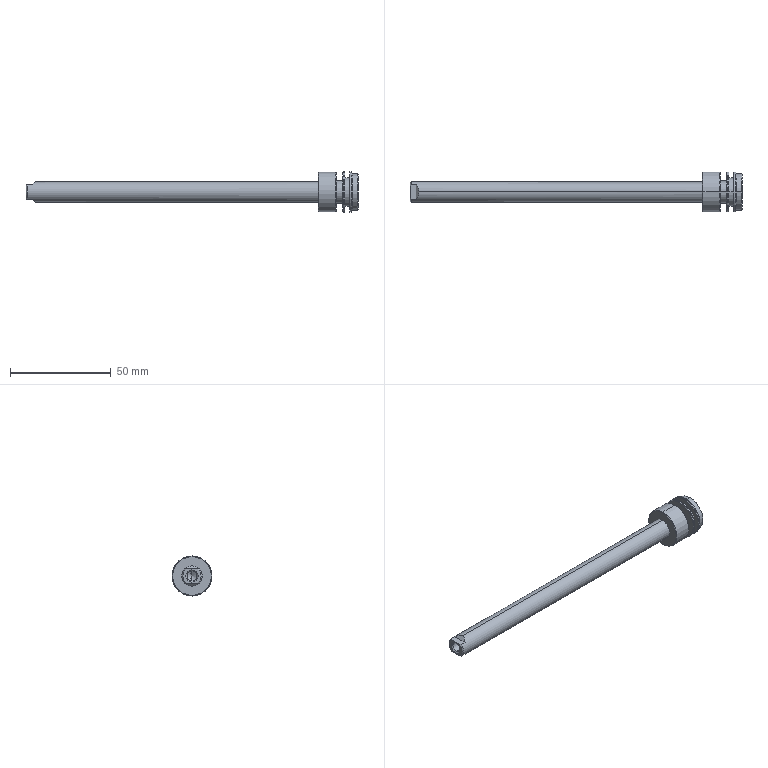Part | STEP file | TC-L-20x125_125r_HI | 1 solid | 49 faces | box 164.5 x 19.9 x 19.9 mm | volume 15852 mm3 | cylinder 16 | cone 14 | plane 11 | torus 8 | commonest cylinder face diameters 19.9 x4 4.917 x2 10 x2 11 x2 14 x2 18 x2